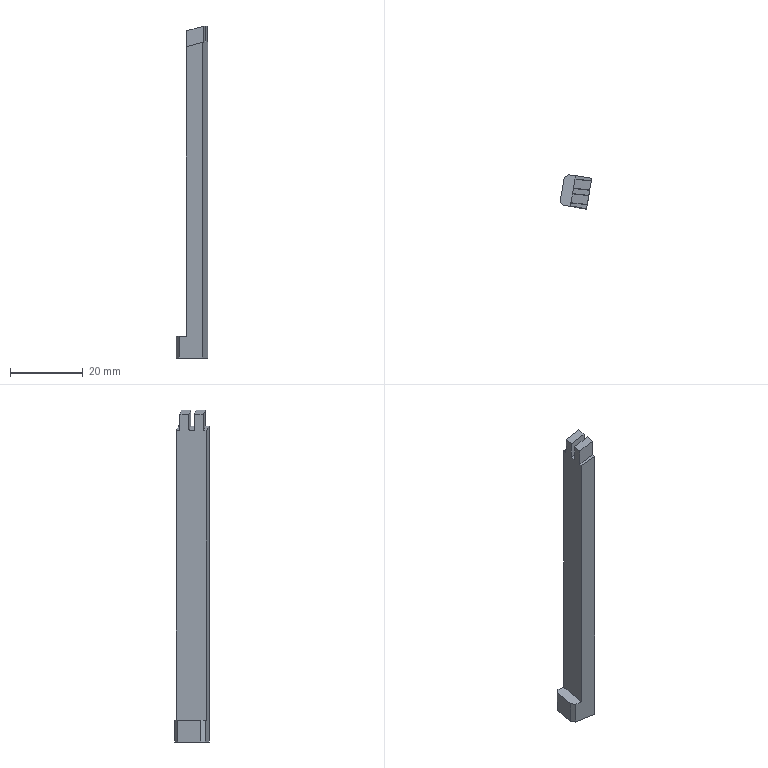Part | STEP file | P011002M016-000 | 1 solid | 18 faces | box 8.688 x 9.5 x 91.429 mm | volume 3552 mm3 | spline 9 | plane 9